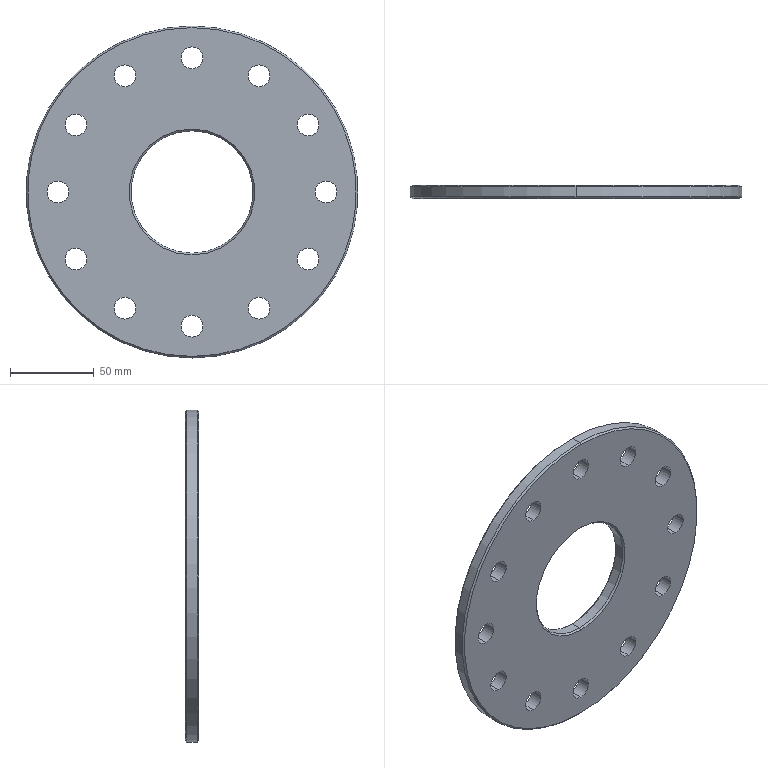Part | SolidWorks | features Chamfer 1, Extrusion 1 | 1 solid | 38 faces | box 198 x 8 x 198 mm | volume 199249 mm3 | cylinder 28 | cone 8 | plane 2 | commonest cylinder face diameters 13 x24 73 x2 198 x2
STEP:
#1=CARTESIAN_POINT('',(0.,79.,-98.));
#2=VERTEX_POINT('',#1);
#3=CARTESIAN_POINT('',(0.,79.,98.));
#4=VERTEX_POINT('',#3);
#5=CARTESIAN_POINT('',(0.,79.,0.));
#6=DIRECTION('',(0.,-1.,0.));
#7=DIRECTION('',(0.,0.,-1.));
#8=AXIS2_PLACEMENT_3D('',#5,#6,#7);
#9=CIRCLE('',#8,98.);
#10=EDGE_CURVE('',#2,#4,#9,.T.);
#11=ORIENTED_EDGE('',*,*,#10,.F.);
#12=CARTESIAN_POINT('',(0.,80.,-99.));
#13=VERTEX_POINT('',#12);
#14=CARTESIAN_POINT('',(0.,80.,-99.));
#15=DIRECTION('',(0.,0.7071,-0.7071));
#16=VECTOR('',#15,1000.);
#17=LINE('',#14,#16);
#18=EDGE_CURVE('',#2,#13,#17,.T.);
#19=ORIENTED_EDGE('',*,*,#18,.T.);
#20=CARTESIAN_POINT('',(0.,80.,99.));
#21=VERTEX_POINT('',#20);
#22=CARTESIAN_POINT('',(0.,80.,0.));
#23=DIRECTION('',(0.,1.,0.));
#24=DIRECTION('',(0.,0.,-1.));
#25=AXIS2_PLACEMENT_3D('',#22,#23,#24);
#26=CIRCLE('',#25,99.);
#27=EDGE_CURVE('',#21,#13,#26,.T.);
#28=ORIENTED_EDGE('',*,*,#27,.F.);
#29=CARTESIAN_POINT('',(0.,80.,99.));
#30=DIRECTION('',(0.,0.7071,0.7071));
#31=VECTOR('',#30,1000.);
#32=LINE('',#29,#31);
#33=EDGE_CURVE('',#4,#21,#32,.T.);
#34=ORIENTED_EDGE('',*,*,#33,.F.);
#35=EDGE_LOOP('',(#11,#19,#28,#34));
#36=FACE_OUTER_BOUND('',#35,.T.);
#37=CARTESIAN_POINT('',(0.,80.,0.));
#38=DIRECTION('',(0.,1.,0.));
#39=DIRECTION('',(0.,0.,1.));
#40=AXIS2_PLACEMENT_3D('',#37,#38,#39);
#41=CONICAL_SURFACE('',#40,99.,0.7854);
#42=ADVANCED_FACE('',(#36),#41,.T.);
#43=CARTESIAN_POINT('',(0.,87.,98.));
#44=VERTEX_POINT('',#43);
#45=CARTESIAN_POINT('',(0.,87.,-98.));
#46=VERTEX_POINT('',#45);
#47=CARTESIAN_POINT('',(0.,87.,0.));
#48=DIRECTION('',(0.,1.,0.));
#49=DIRECTION('',(0.,0.,-1.));
#50=AXIS2_PLACEMENT_3D('',#47,#48,#49);
#51=CIRCLE('',#50,98.);
#52=EDGE_CURVE('',#44,#46,#51,.T.);
#53=ORIENTED_EDGE('',*,*,#52,.F.);
#54=CARTESIAN_POINT('',(0.,86.,99.));
#55=VERTEX_POINT('',#54);
#56=CARTESIAN_POINT('',(0.,87.,98.));
#57=DIRECTION('',(0.,-0.7071,0.7071));
#58=VECTOR('',#57,1000.);
#59=LINE('',#56,#58);
#60=EDGE_CURVE('',#44,#55,#59,.T.);
#61=ORIENTED_EDGE('',*,*,#60,.T.);
#62=CARTESIAN_POINT('',(0.,86.,-99.));
#63=VERTEX_POINT('',#62);
#64=CARTESIAN_POINT('',(0.,86.,0.));
#65=DIRECTION('',(0.,-1.,0.));
#66=DIRECTION('',(0.,0.,-1.));
#67=AXIS2_PLACEMENT_3D('',#64,#65,#66);
#68=CIRCLE('',#67,99.);
#69=EDGE_CURVE('',#63,#55,#68,.T.);
#70=ORIENTED_EDGE('',*,*,#69,.F.);
#71=CARTESIAN_POINT('',(0.,87.,-98.));
#72=DIRECTION('',(0.,-0.7071,-0.7071));
#73=VECTOR('',#72,1000.);
#74=LINE('',#71,#73);
#75=EDGE_CURVE('',#46,#63,#74,.T.);
#76=ORIENTED_EDGE('',*,*,#75,.F.);
#77=EDGE_LOOP('',(#53,#61,#70,#76));
#78=FACE_OUTER_BOUND('',#77,.T.);
#79=CARTESIAN_POINT('',(0.,87.,0.));
#80=DIRECTION('',(0.,-1.,0.));
#81=DIRECTION('',(0.,0.,-1.));
#82=AXIS2_PLACEMENT_3D('',#79,#80,#81);
#83=CONICAL_SURFACE('',#82,98.,0.7854);
#84=ADVANCED_FACE('',(#78),#83,.T.);
#85=CARTESIAN_POINT('',(0.,80.,36.5));
#86=VERTEX_POINT('',#85);
#87=CARTESIAN_POINT('',(0.,80.,-36.5));
#88=VERTEX_POINT('',#87);
#89=CARTESIAN_POINT('',(0.,80.,0.));
#90=DIRECTION('',(0.,-1.,0.));
#91=DIRECTION('',(0.,0.,-1.));
#92=AXIS2_PLACEMENT_3D('',#89,#90,#91);
#93=CIRCLE('',#92,36.5);
#94=EDGE_CURVE('',#86,#88,#93,.T.);
#95=ORIENTED_EDGE('',*,*,#94,.F.);
#96=CARTESIAN_POINT('',(0.,79.,37.5));
#97=VERTEX_POINT('',#96);
#98=CARTESIAN_POINT('',(0.,79.,37.5));
#99=DIRECTION('',(0.,-0.7071,0.7071));
#100=VECTOR('',#99,1000.);
#101=LINE('',#98,#100);
#102=EDGE_CURVE('',#86,#97,#101,.T.);
#103=ORIENTED_EDGE('',*,*,#102,.T.);
#104=CARTESIAN_POINT('',(0.,79.,-37.5));
#105=VERTEX_POINT('',#104);
#106=CARTESIAN_POINT('',(0.,79.,0.));
#107=DIRECTION('',(0.,1.,0.));
#108=DIRECTION('',(0.,0.,-1.));
#109=AXIS2_PLACEMENT_3D('',#106,#107,#108);
#110=CIRCLE('',#109,37.5);
#111=EDGE_CURVE('',#105,#97,#110,.T.);
#112=ORIENTED_EDGE('',*,*,#111,.F.);
#113=CARTESIAN_POINT('',(0.,79.,-37.5));
#114=DIRECTION('',(0.,-0.7071,-0.7071));
#115=VECTOR('',#114,1000.);
#116=LINE('',#113,#115);
#117=EDGE_CURVE('',#88,#105,#116,.T.);
#118=ORIENTED_EDGE('',*,*,#117,.F.);
#119=EDGE_LOOP('',(#95,#103,#112,#118));
#120=FACE_OUTER_BOUND('',#119,.T.);
#121=CARTESIAN_POINT('',(0.,79.,0.));
#122=DIRECTION('',(0.,-1.,0.));
#123=DIRECTION('',(0.,0.,-1.));
#124=AXIS2_PLACEMENT_3D('',#121,#122,#123);
#125=CONICAL_SURFACE('',#124,37.5,0.7854);
#126=ADVANCED_FACE('',(#120),#125,.F.);
#127=CARTESIAN_POINT('',(0.,86.,-36.5));
#128=VERTEX_POINT('',#127);
#129=CARTESIAN_POINT('',(0.,86.,36.5));
#130=VERTEX_POINT('',#129);
#131=CARTESIAN_POINT('',(0.,86.,0.));
#132=DIRECTION('',(0.,1.,0.));
#133=DIRECTION('',(0.,0.,-1.));
#134=AXIS2_PLACEMENT_3D('',#131,#132,#133);
#135=CIRCLE('',#134,36.5);
#136=EDGE_CURVE('',#128,#130,#135,.T.);
#137=ORIENTED_EDGE('',*,*,#136,.F.);
#138=CARTESIAN_POINT('',(0.,87.,-37.5));
#139=VERTEX_POINT('',#138);
#140=CARTESIAN_POINT('',(0.,86.,-36.5));
#141=DIRECTION('',(0.,0.7071,-0.7071));
#142=VECTOR('',#141,1000.);
#143=LINE('',#140,#142);
#144=EDGE_CURVE('',#128,#139,#143,.T.);
#145=ORIENTED_EDGE('',*,*,#144,.T.);
#146=CARTESIAN_POINT('',(0.,87.,37.5));
#147=VERTEX_POINT('',#146);
#148=CARTESIAN_POINT('',(0.,87.,0.));
#149=DIRECTION('',(0.,-1.,0.));
#150=DIRECTION('',(0.,0.,-1.));
#151=AXIS2_PLACEMENT_3D('',#148,#149,#150);
#152=CIRCLE('',#151,37.5);
#153=EDGE_CURVE('',#147,#139,#152,.T.);
#154=ORIENTED_EDGE('',*,*,#153,.F.);
#155=CARTESIAN_POINT('',(0.,86.,36.5));
#156=DIRECTION('',(0.,0.7071,0.7071));
#157=VECTOR('',#156,1000.);
#158=LINE('',#155,#157);
#159=EDGE_CURVE('',#130,#147,#158,.T.);
#160=ORIENTED_EDGE('',*,*,#159,.F.);
#161=EDGE_LOOP('',(#137,#145,#154,#160));
#162=FACE_OUTER_BOUND('',#161,.T.);
#163=CARTESIAN_POINT('',(0.,86.,0.));
#164=DIRECTION('',(0.,1.,0.));
#165=DIRECTION('',(0.,0.,1.));
#166=AXIS2_PLACEMENT_3D('',#163,#164,#165);
#167=CONICAL_SURFACE('',#166,36.5,0.7854);
#168=ADVANCED_FACE('',(#162),#167,.F.);
#169=ORIENTED_EDGE('',*,*,#94,.T.);
#170=CARTESIAN_POINT('',(0.,79.,-36.5));
#171=DIRECTION('',(0.,1.,0.));
#172=VECTOR('',#171,1000.);
#173=LINE('',#170,#172);
#174=EDGE_CURVE('',#88,#128,#173,.T.);
#175=ORIENTED_EDGE('',*,*,#174,.T.);
#176=ORIENTED_EDGE('',*,*,#136,.T.);
#177=CARTESIAN_POINT('',(0.,79.,36.5));
#178=DIRECTION('',(0.,1.,0.));
#179=VECTOR('',#178,1000.);
#180=LINE('',#177,#179);
#181=EDGE_CURVE('',#86,#130,#180,.T.);
#182=ORIENTED_EDGE('',*,*,#181,.F.);
#183=EDGE_LOOP('',(#169,#175,#176,#182));
#184=FACE_OUTER_BOUND('',#183,.T.);
#185=CARTESIAN_POINT('',(0.,79.,0.));
#186=DIRECTION('',(0.,1.,0.));
#187=DIRECTION('',(0.,0.,1.));
#188=AXIS2_PLACEMENT_3D('',#185,#186,#187);
#189=CYLINDRICAL_SURFACE('',#188,36.5);
#190=ADVANCED_FACE('',(#184),#189,.F.);
#191=CARTESIAN_POINT('',(80.,79.,-6.5));
#192=VERTEX_POINT('',#191);
#193=CARTESIAN_POINT('',(80.,79.,6.5));
#194=VERTEX_POINT('',#193);
#195=CARTESIAN_POINT('',(80.,79.,0.));
#196=DIRECTION('',(0.,1.,0.));
#197=DIRECTION('',(0.,0.,-1.));
#198=AXIS2_PLACEMENT_3D('',#195,#196,#197);
#199=CIRCLE('',#198,6.5);
#200=EDGE_CURVE('',#192,#194,#199,.T.);
#201=ORIENTED_EDGE('',*,*,#200,.F.);
#202=CARTESIAN_POINT('',(80.,87.,-6.5));
#203=VERTEX_POINT('',#202);
#204=CARTESIAN_POINT('',(80.,79.,-6.5));
#205=DIRECTION('',(0.,1.,0.));
#206=VECTOR('',#205,1000.);
#207=LINE('',#204,#206);
#208=EDGE_CURVE('',#192,#203,#207,.T.);
#209=ORIENTED_EDGE('',*,*,#208,.T.);
#210=CARTESIAN_POINT('',(80.,87.,6.5));
#211=VERTEX_POINT('',#210);
#212=CARTESIAN_POINT('',(80.,87.,0.));
#213=DIRECTION('',(0.,1.,0.));
#214=DIRECTION('',(0.,0.,-1.));
#215=AXIS2_PLACEMENT_3D('',#212,#213,#214);
#216=CIRCLE('',#215,6.5);
#217=EDGE_CURVE('',#203,#211,#216,.T.);
#218=ORIENTED_EDGE('',*,*,#217,.T.);
#219=CARTESIAN_POINT('',(80.,79.,6.5));
#220=DIRECTION('',(0.,1.,0.));
#221=VECTOR('',#220,1000.);
#222=LINE('',#219,#221);
#223=EDGE_CURVE('',#194,#211,#222,.T.);
#224=ORIENTED_EDGE('',*,*,#223,.F.);
#225=EDGE_LOOP('',(#201,#209,#218,#224));
#226=FACE_OUTER_BOUND('',#225,.T.);
#227=CARTESIAN_POINT('',(80.,79.,0.));
#228=DIRECTION('',(0.,1.,0.));
#229=DIRECTION('',(0.,0.,1.));
#230=AXIS2_PLACEMENT_3D('',#227,#228,#229);
#231=CYLINDRICAL_SURFACE('',#230,6.5);
#232=ADVANCED_FACE('',(#226),#231,.F.);
#233=CARTESIAN_POINT('',(-40.,79.,62.782));
#234=VERTEX_POINT('',#233);
#235=CARTESIAN_POINT('',(-40.,79.,75.782));
#236=VERTEX_POINT('',#235);
#237=CARTESIAN_POINT('',(-40.,79.,69.282));
#238=DIRECTION('',(0.,1.,0.));
#239=DIRECTION('',(0.,0.,-1.));
#240=AXIS2_PLACEMENT_3D('',#237,#238,#239);
#241=CIRCLE('',#240,6.5);
#242=EDGE_CURVE('',#234,#236,#241,.T.);
#243=ORIENTED_EDGE('',*,*,#242,.F.);
#244=CARTESIAN_POINT('',(-40.,87.,62.782));
#245=VERTEX_POINT('',#244);
#246=CARTESIAN_POINT('',(-40.,79.,62.782));
#247=DIRECTION('',(0.,1.,0.));
#248=VECTOR('',#247,1000.);
#249=LINE('',#246,#248);
#250=EDGE_CURVE('',#234,#245,#249,.T.);
#251=ORIENTED_EDGE('',*,*,#250,.T.);
#252=CARTESIAN_POINT('',(-40.,87.,75.782));
#253=VERTEX_POINT('',#252);
#254=CARTESIAN_POINT('',(-40.,87.,69.282));
#255=DIRECTION('',(0.,1.,0.));
#256=DIRECTION('',(0.,0.,-1.));
#257=AXIS2_PLACEMENT_3D('',#254,#255,#256);
#258=CIRCLE('',#257,6.5);
#259=EDGE_CURVE('',#245,#253,#258,.T.);
#260=ORIENTED_EDGE('',*,*,#259,.T.);
#261=CARTESIAN_POINT('',(-40.,79.,75.782));
#262=DIRECTION('',(0.,1.,0.));
#263=VECTOR('',#262,1000.);
#264=LINE('',#261,#263);
#265=EDGE_CURVE('',#236,#253,#264,.T.);
#266=ORIENTED_EDGE('',*,*,#265,.F.);
#267=EDGE_LOOP('',(#243,#251,#260,#266));
#268=FACE_OUTER_BOUND('',#267,.T.);
#269=CARTESIAN_POINT('',(-40.,79.,69.282));
#270=DIRECTION('',(0.,1.,0.));
#271=DIRECTION('',(0.,0.,1.));
#272=AXIS2_PLACEMENT_3D('',#269,#270,#271);
#273=CYLINDRICAL_SURFACE('',#272,6.5);
#274=ADVANCED_FACE('',(#268),#273,.F.);
#275=CARTESIAN_POINT('',(69.282,79.,-46.5));
#276=VERTEX_POINT('',#275);
#277=CARTESIAN_POINT('',(69.282,79.,-33.5));
#278=VERTEX_POINT('',#277);
#279=CARTESIAN_POINT('',(69.282,79.,-40.));
#280=DIRECTION('',(0.,1.,0.));
#281=DIRECTION('',(0.,0.,-1.));
#282=AXIS2_PLACEMENT_3D('',#279,#280,#281);
#283=CIRCLE('',#282,6.5);
#284=EDGE_CURVE('',#276,#278,#283,.T.);
#285=ORIENTED_EDGE('',*,*,#284,.F.);
#286=CARTESIAN_POINT('',(69.282,87.,-46.5));
#287=VERTEX_POINT('',#286);
#288=CARTESIAN_POINT('',(69.282,79.,-46.5));
#289=DIRECTION('',(0.,1.,0.));
#290=VECTOR('',#289,1000.);
#291=LINE('',#288,#290);
#292=EDGE_CURVE('',#276,#287,#291,.T.);
#293=ORIENTED_EDGE('',*,*,#292,.T.);
#294=CARTESIAN_POINT('',(69.282,87.,-33.5));
#295=VERTEX_POINT('',#294);
#296=CARTESIAN_POINT('',(69.282,87.,-40.));
#297=DIRECTION('',(0.,1.,0.));
#298=DIRECTION('',(0.,0.,-1.));
#299=AXIS2_PLACEMENT_3D('',#296,#297,#298);
#300=CIRCLE('',#299,6.5);
#301=EDGE_CURVE('',#287,#295,#300,.T.);
#302=ORIENTED_EDGE('',*,*,#301,.T.);
#303=CARTESIAN_POINT('',(69.282,79.,-33.5));
#304=DIRECTION('',(0.,1.,0.));
#305=VECTOR('',#304,1000.);
#306=LINE('',#303,#305);
#307=EDGE_CURVE('',#278,#295,#306,.T.);
#308=ORIENTED_EDGE('',*,*,#307,.F.);
#309=EDGE_LOOP('',(#285,#293,#302,#308));
#310=FACE_OUTER_BOUND('',#309,.T.);
#311=CARTESIAN_POINT('',(69.282,79.,-40.));
#312=DIRECTION('',(0.,1.,0.));
#313=DIRECTION('',(0.,0.,1.));
#314=AXIS2_PLACEMENT_3D('',#311,#312,#313);
#315=CYLINDRICAL_SURFACE('',#314,6.5);
#316=ADVANCED_FACE('',(#310),#315,.F.);
#317=CARTESIAN_POINT('',(40.,79.,62.782));
#318=VERTEX_POINT('',#317);
#319=CARTESIAN_POINT('',(40.,79.,75.782));
#320=VERTEX_POINT('',#319);
#321=CARTESIAN_POINT('',(40.,79.,69.282));
#322=DIRECTION('',(0.,1.,0.));
#323=DIRECTION('',(0.,0.,-1.));
#324=AXIS2_PLACEMENT_3D('',#321,#322,#323);
#325=CIRCLE('',#324,6.5);
#326=EDGE_CURVE('',#318,#320,#325,.T.);
#327=ORIENTED_EDGE('',*,*,#326,.F.);
#328=CARTESIAN_POINT('',(40.,87.,62.782));
#329=VERTEX_POINT('',#328);
#330=CARTESIAN_POINT('',(40.,79.,62.782));
#331=DIRECTION('',(0.,1.,0.));
#332=VECTOR('',#331,1000.);
#333=LINE('',#330,#332);
#334=EDGE_CURVE('',#318,#329,#333,.T.);
#335=ORIENTED_EDGE('',*,*,#334,.T.);
#336=CARTESIAN_POINT('',(40.,87.,75.782));
#337=VERTEX_POINT('',#336);
#338=CARTESIAN_POINT('',(40.,87.,69.282));
#339=DIRECTION('',(0.,1.,0.));
#340=DIRECTION('',(0.,0.,-1.));
#341=AXIS2_PLACEMENT_3D('',#338,#339,#340);
#342=CIRCLE('',#341,6.5);
#343=EDGE_CURVE('',#329,#337,#342,.T.);
#344=ORIENTED_EDGE('',*,*,#343,.T.);
#345=CARTESIAN_POINT('',(40.,79.,75.782));
#346=DIRECTION('',(0.,1.,0.));
#347=VECTOR('',#346,1000.);
#348=LINE('',#345,#347);
#349=EDGE_CURVE('',#320,#337,#348,.T.);
#350=ORIENTED_EDGE('',*,*,#349,.F.);
#351=EDGE_LOOP('',(#327,#335,#344,#350));
#352=FACE_OUTER_BOUND('',#351,.T.);
#353=CARTESIAN_POINT('',(40.,79.,69.282));
#354=DIRECTION('',(0.,1.,0.));
#355=DIRECTION('',(0.,0.,1.));
#356=AXIS2_PLACEMENT_3D('',#353,#354,#355);
#357=CYLINDRICAL_SURFACE('',#356,6.5);
#358=ADVANCED_FACE('',(#352),#357,.F.);
#359=CARTESIAN_POINT('',(0.,79.,73.5));
#360=VERTEX_POINT('',#359);
#361=CARTESIAN_POINT('',(0.,79.,86.5));
#362=VERTEX_POINT('',#361);
#363=CARTESIAN_POINT('',(0.,79.,80.));
#364=DIRECTION('',(0.,1.,0.));
#365=DIRECTION('',(0.,0.,-1.));
#366=AXIS2_PLACEMENT_3D('',#363,#364,#365);
#367=CIRCLE('',#366,6.5);
#368=EDGE_CURVE('',#360,#362,#367,.T.);
#369=ORIENTED_EDGE('',*,*,#368,.F.);
#370=CARTESIAN_POINT('',(0.,87.,73.5));
#371=VERTEX_POINT('',#370);
#372=CARTESIAN_POINT('',(0.,79.,73.5));
#373=DIRECTION('',(0.,1.,0.));
#374=VECTOR('',#373,1000.);
#375=LINE('',#372,#374);
#376=EDGE_CURVE('',#360,#371,#375,.T.);
#377=ORIENTED_EDGE('',*,*,#376,.T.);
#378=CARTESIAN_POINT('',(0.,87.,86.5));
#379=VERTEX_POINT('',#378);
#380=CARTESIAN_POINT('',(0.,87.,80.));
#381=DIRECTION('',(0.,1.,0.));
#382=DIRECTION('',(0.,0.,-1.));
#383=AXIS2_PLACEMENT_3D('',#380,#381,#382);
#384=CIRCLE('',#383,6.5);
#385=EDGE_CURVE('',#371,#379,#384,.T.);
#386=ORIENTED_EDGE('',*,*,#385,.T.);
#387=CARTESIAN_POINT('',(0.,79.,86.5));
#388=DIRECTION('',(0.,1.,0.));
#389=VECTOR('',#388,1000.);
#390=LINE('',#387,#389);
#391=EDGE_CURVE('',#362,#379,#390,.T.);
#392=ORIENTED_EDGE('',*,*,#391,.F.);
#393=EDGE_LOOP('',(#369,#377,#386,#392));
#394=FACE_OUTER_BOUND('',#393,.T.);
#395=CARTESIAN_POINT('',(0.,79.,80.));
#396=DIRECTION('',(0.,1.,0.));
#397=DIRECTION('',(0.,0.,1.));
#398=AXIS2_PLACEMENT_3D('',#395,#396,#397);
#399=CYLINDRICAL_SURFACE('',#398,6.5);
#400=ADVANCED_FACE('',(#394),#399,.F.);
#401=CARTESIAN_POINT('',(-40.,79.,-75.782));
#402=VERTEX_POINT('',#401);
#403=CARTESIAN_POINT('',(-40.,79.,-62.782));
#404=VERTEX_POINT('',#403);
#405=CARTESIAN_POINT('',(-40.,79.,-69.282));
#406=DIRECTION('',(0.,1.,0.));
#407=DIRECTION('',(0.,0.,-1.));
#408=AXIS2_PLACEMENT_3D('',#405,#406,#407);
#409=CIRCLE('',#408,6.5);
#410=EDGE_CURVE('',#402,#404,#409,.T.);
#411=ORIENTED_EDGE('',*,*,#410,.F.);
#412=CARTESIAN_POINT('',(-40.,87.,-75.782));
#413=VERTEX_POINT('',#412);
#414=CARTESIAN_POINT('',(-40.,79.,-75.782));
#415=DIRECTION('',(0.,1.,0.));
#416=VECTOR('',#415,1000.);
#417=LINE('',#414,#416);
#418=EDGE_CURVE('',#402,#413,#417,.T.);
#419=ORIENTED_EDGE('',*,*,#418,.T.);
#420=CARTESIAN_POINT('',(-40.,87.,-62.782));
#421=VERTEX_POINT('',#420);
#422=CARTESIAN_POINT('',(-40.,87.,-69.282));
#423=DIRECTION('',(0.,1.,0.));
#424=DIRECTION('',(0.,0.,-1.));
#425=AXIS2_PLACEMENT_3D('',#422,#423,#424);
#426=CIRCLE('',#425,6.5);
#427=EDGE_CURVE('',#413,#421,#426,.T.);
#428=ORIENTED_EDGE('',*,*,#427,.T.);
#429=CARTESIAN_POINT('',(-40.,79.,-62.782));
#430=DIRECTION('',(0.,1.,0.));
#431=VECTOR('',#430,1000.);
#432=LINE('',#429,#431);
#433=EDGE_CURVE('',#404,#421,#432,.T.);
#434=ORIENTED_EDGE('',*,*,#433,.F.);
#435=EDGE_LOOP('',(#411,#419,#428,#434));
#436=FACE_OUTER_BOUND('',#435,.T.);
#437=CARTESIAN_POINT('',(-40.,79.,-69.282));
#438=DIRECTION('',(0.,1.,0.));
#439=DIRECTION('',(0.,0.,1.));
#440=AXIS2_PLACEMENT_3D('',#437,#438,#439);
#441=CYLINDRICAL_SURFACE('',#440,6.5);
#442=ADVANCED_FACE('',(#436),#441,.F.);
#443=CARTESIAN_POINT('',(69.282,79.,33.5));
#444=VERTEX_POINT('',#443);
#445=CARTESIAN_POINT('',(69.282,79.,46.5));
#446=VERTEX_POINT('',#445);
#447=CARTESIAN_POINT('',(69.282,79.,40.));
#448=DIRECTION('',(0.,1.,0.));
#449=DIRECTION('',(0.,0.,-1.));
#450=AXIS2_PLACEMENT_3D('',#447,#448,#449);
#451=CIRCLE('',#450,6.5);
#452=EDGE_CURVE('',#444,#446,#451,.T.);
#453=ORIENTED_EDGE('',*,*,#452,.F.);
#454=CARTESIAN_POINT('',(69.282,87.,33.5));
#455=VERTEX_POINT('',#454);
#456=CARTESIAN_POINT('',(69.282,79.,33.5));
#457=DIRECTION('',(0.,1.,0.));
#458=VECTOR('',#457,1000.);
#459=LINE('',#456,#458);
#460=EDGE_CURVE('',#444,#455,#459,.T.);
#461=ORIENTED_EDGE('',*,*,#460,.T.);
#462=CARTESIAN_POINT('',(69.282,87.,46.5));
#463=VERTEX_POINT('',#462);
#464=CARTESIAN_POINT('',(69.282,87.,40.));
#465=DIRECTION('',(0.,1.,0.));
#466=DIRECTION('',(0.,0.,-1.));
#467=AXIS2_PLACEMENT_3D('',#464,#465,#466);
#468=CIRCLE('',#467,6.5);
#469=EDGE_CURVE('',#455,#463,#468,.T.);
#470=ORIENTED_EDGE('',*,*,#469,.T.);
#471=CARTESIAN_POINT('',(69.282,79.,46.5));
#472=DIRECTION('',(0.,1.,0.));
#473=VECTOR('',#472,1000.);
#474=LINE('',#471,#473);
#475=EDGE_CURVE('',#446,#463,#474,.T.);
#476=ORIENTED_EDGE('',*,*,#475,.F.);
#477=EDGE_LOOP('',(#453,#461,#470,#476));
#478=FACE_OUTER_BOUND('',#477,.T.);
#479=CARTESIAN_POINT('',(69.282,79.,40.));
#480=DIRECTION('',(0.,1.,0.));
#481=DIRECTION('',(0.,0.,1.));
#482=AXIS2_PLACEMENT_3D('',#479,#480,#481);
#483=CYLINDRICAL_SURFACE('',#482,6.5);
#484=ADVANCED_FACE('',(#478),#483,.F.);
#485=CARTESIAN_POINT('',(0.,79.,-86.5));
#486=VERTEX_POINT('',#485);
#487=CARTESIAN_POINT('',(0.,79.,-73.5));
#488=VERTEX_POINT('',#487);
#489=CARTESIAN_POINT('',(0.,79.,-80.));
#490=DIRECTION('',(0.,1.,0.));
#491=DIRECTION('',(0.,0.,-1.));
#492=AXIS2_PLACEMENT_3D('',#489,#490,#491);
#493=CIRCLE('',#492,6.5);
#494=EDGE_CURVE('',#486,#488,#493,.T.);
#495=ORIENTED_EDGE('',*,*,#494,.F.);
#496=CARTESIAN_POINT('',(0.,87.,-86.5));
#497=VERTEX_POINT('',#496);
#498=CARTESIAN_POINT('',(0.,79.,-86.5));
#499=DIRECTION('',(0.,1.,0.));
#500=VECTOR('',#499,1000.);
#501=LINE('',#498,#500);
#502=EDGE_CURVE('',#486,#497,#501,.T.);
#503=ORIENTED_EDGE('',*,*,#502,.T.);
#504=CARTESIAN_POINT('',(0.,87.,-73.5));
#505=VERTEX_POINT('',#504);
#506=CARTESIAN_POINT('',(0.,87.,-80.));
#507=DIRECTION('',(0.,1.,0.));
#508=DIRECTION('',(0.,0.,-1.));
#509=AXIS2_PLACEMENT_3D('',#506,#507,#508);
#510=CIRCLE('',#509,6.5);
#511=EDGE_CURVE('',#497,#505,#510,.T.);
#512=ORIENTED_EDGE('',*,*,#511,.T.);
#513=CARTESIAN_POINT('',(0.,79.,-73.5));
#514=DIRECTION('',(0.,1.,0.));
#515=VECTOR('',#514,1000.);
#516=LINE('',#513,#515);
#517=EDGE_CURVE('',#488,#505,#516,.T.);
#518=ORIENTED_EDGE('',*,*,#517,.F.);
#519=EDGE_LOOP('',(#495,#503,#512,#518));
#520=FACE_OUTER_BOUND('',#519,.T.);
#521=CARTESIAN_POINT('',(0.,79.,-80.));
#522=DIRECTION('',(0.,1.,0.));
#523=DIRECTION('',(0.,0.,1.));
#524=AXIS2_PLACEMENT_3D('',#521,#522,#523);
#525=CYLINDRICAL_SURFACE('',#524,6.5);
#526=ADVANCED_FACE('',(#520),#525,.F.);
#527=CARTESIAN_POINT('',(-69.282,79.,33.5));
#528=VERTEX_POINT('',#527);
#529=CARTESIAN_POINT('',(-69.282,79.,46.5));
#530=VERTEX_POINT('',#529);
#531=CARTESIAN_POINT('',(-69.282,79.,40.));
#532=DIRECTION('',(0.,1.,0.));
#533=DIRECTION('',(0.,0.,-1.));
#534=AXIS2_PLACEMENT_3D('',#531,#532,#533);
#535=CIRCLE('',#534,6.5);
#536=EDGE_CURVE('',#528,#530,#535,.T.);
#537=ORIENTED_EDGE('',*,*,#536,.F.);
#538=CARTESIAN_POINT('',(-69.282,87.,33.5));
#539=VERTEX_POINT('',#538);
#540=CARTESIAN_POINT('',(-69.282,79.,33.5));
#541=DIRECTION('',(0.,1.,0.));
#542=VECTOR('',#541,1000.);
#543=LINE('',#540,#542);
#544=EDGE_CURVE('',#528,#539,#543,.T.);
#545=ORIENTED_EDGE('',*,*,#544,.T.);
#546=CARTESIAN_POINT('',(-69.282,87.,46.5));
#547=VERTEX_POINT('',#546);
#548=CARTESIAN_POINT('',(-69.282,87.,40.));
#549=DIRECTION('',(0.,1.,0.));
#550=DIRECTION('',(0.,0.,-1.));
#551=AXIS2_PLACEMENT_3D('',#548,#549,#550);
#552=CIRCLE('',#551,6.5);
#553=EDGE_CURVE('',#539,#547,#552,.T.);
#554=ORIENTED_EDGE('',*,*,#553,.T.);
#555=CARTESIAN_POINT('',(-69.282,79.,46.5));
#556=DIRECTION('',(0.,1.,0.));
#557=VECTOR('',#556,1000.);
#558=LINE('',#555,#557);
#559=EDGE_CURVE('',#530,#547,#558,.T.);
#560=ORIENTED_EDGE('',*,*,#559,.F.);
#561=EDGE_LOOP('',(#537,#545,#554,#560));
#562=FACE_OUTER_BOUND('',#561,.T.);
#563=CARTESIAN_POINT('',(-69.282,79.,40.));
#564=DIRECTION('',(0.,1.,0.));
#565=DIRECTION('',(0.,0.,1.));
#566=AXIS2_PLACEMENT_3D('',#563,#564,#565);
#567=CYLINDRICAL_SURFACE('',#566,6.5);
#568=ADVANCED_FACE('',(#562),#567,.F.);
#569=CARTESIAN_POINT('',(-69.282,79.,-46.5));
#570=VERTEX_POINT('',#569);
#571=CARTESIAN_POINT('',(-69.282,79.,-33.5));
#572=VERTEX_POINT('',#571);
#573=CARTESIAN_POINT('',(-69.282,79.,-40.));
#574=DIRECTION('',(0.,1.,0.));
#575=DIRECTION('',(0.,0.,-1.));
#576=AXIS2_PLACEMENT_3D('',#573,#574,#575);
#577=CIRCLE('',#576,6.5);
#578=EDGE_CURVE('',#570,#572,#577,.T.);
#579=ORIENTED_EDGE('',*,*,#578,.F.);
#580=CARTESIAN_POINT('',(-69.282,87.,-46.5));
#581=VERTEX_POINT('',#580);
#582=CARTESIAN_POINT('',(-69.282,79.,-46.5));
#583=DIRECTION('',(0.,1.,0.));
#584=VECTOR('',#583,1000.);
#585=LINE('',#582,#584);
#586=EDGE_CURVE('',#570,#581,#585,.T.);
#587=ORIENTED_EDGE('',*,*,#586,.T.);
#588=CARTESIAN_POINT('',(-69.282,87.,-33.5));
#589=VERTEX_POINT('',#588);
#590=CARTESIAN_POINT('',(-69.282,87.,-40.));
#591=DIRECTION('',(0.,1.,0.));
#592=DIRECTION('',(0.,0.,-1.));
#593=AXIS2_PLACEMENT_3D('',#590,#591,#592);
#594=CIRCLE('',#593,6.5);
#595=EDGE_CURVE('',#581,#589,#594,.T.);
#596=ORIENTED_EDGE('',*,*,#595,.T.);
#597=CARTESIAN_POINT('',(-69.282,79.,-33.5));
#598=DIRECTION('',(0.,1.,0.));
#599=VECTOR('',#598,1000.);
#600=LINE('',#597,#599);
#601=EDGE_CURVE('',#572,#589,#600,.T.);
#602=ORIENTED_EDGE('',*,*,#601,.F.);
#603=EDGE_LOOP('',(#579,#587,#596,#602));
#604=FACE_OUTER_BOUND('',#603,.T.);
#605=CARTESIAN_POINT('',(-69.282,79.,-40.));
#606=DIRECTION('',(0.,1.,0.));
#607=DIRECTION('',(0.,0.,1.));
#608=AXIS2_PLACEMENT_3D('',#605,#606,#607);
#609=CYLINDRICAL_SURFACE('',#608,6.5);
#610=ADVANCED_FACE('',(#604),#609,.F.);
#611=CARTESIAN_POINT('',(40.,79.,-75.782));
#612=VERTEX_POINT('',#611);
#613=CARTESIAN_POINT('',(40.,79.,-62.782));
#614=VERTEX_POINT('',#613);
#615=CARTESIAN_POINT('',(40.,79.,-69.282));
#616=DIRECTION('',(0.,1.,0.));
#617=DIRECTION('',(0.,0.,-1.));
#618=AXIS2_PLACEMENT_3D('',#615,#616,#617);
#619=CIRCLE('',#618,6.5);
#620=EDGE_CURVE('',#612,#614,#619,.T.);
#621=ORIENTED_EDGE('',*,*,#620,.F.);
#622=CARTESIAN_POINT('',(40.,87.,-75.782));
#623=VERTEX_POINT('',#622);
#624=CARTESIAN_POINT('',(40.,79.,-75.782));
#625=DIRECTION('',(0.,1.,0.));
#626=VECTOR('',#625,1000.);
#627=LINE('',#624,#626);
#628=EDGE_CURVE('',#612,#623,#627,.T.);
#629=ORIENTED_EDGE('',*,*,#628,.T.);
#630=CARTESIAN_POINT('',(40.,87.,-62.782));
#631=VERTEX_POINT('',#630);
#632=CARTESIAN_POINT('',(40.,87.,-69.282));
#633=DIRECTION('',(0.,1.,0.));
#634=DIRECTION('',(0.,0.,-1.));
#635=AXIS2_PLACEMENT_3D('',#632,#633,#634);
#636=CIRCLE('',#635,6.5);
#637=EDGE_CURVE('',#623,#631,#636,.T.);
#638=ORIENTED_EDGE('',*,*,#637,.T.);
#639=CARTESIAN_POINT('',(40.,79.,-62.782));
#640=DIRECTION('',(0.,1.,0.));
#641=VECTOR('',#640,1000.);
#642=LINE('',#639,#641);
#643=EDGE_CURVE('',#614,#631,#642,.T.);
#644=ORIENTED_EDGE('',*,*,#643,.F.);
#645=EDGE_LOOP('',(#621,#629,#638,#644));
#646=FACE_OUTER_BOUND('',#645,.T.);
#647=CARTESIAN_POINT('',(40.,79.,-69.282));
#648=DIRECTION('',(0.,1.,0.));
#649=DIRECTION('',(0.,0.,1.));
#650=AXIS2_PLACEMENT_3D('',#647,#648,#649);
#651=CYLINDRICAL_SURFACE('',#650,6.5);
#652=ADVANCED_FACE('',(#646),#651,.F.);
#653=CARTESIAN_POINT('',(-80.,79.,-6.5));
#654=VERTEX_POINT('',#653);
#655=CARTESIAN_POINT('',(-80.,79.,6.5));
#656=VERTEX_POINT('',#655);
#657=CARTESIAN_POINT('',(-80.,79.,0.));
#658=DIRECTION('',(0.,1.,0.));
#659=DIRECTION('',(0.,0.,-1.));
#660=AXIS2_PLACEMENT_3D('',#657,#658,#659);
#661=CIRCLE('',#660,6.5);
#662=EDGE_CURVE('',#654,#656,#661,.T.);
#663=ORIENTED_EDGE('',*,*,#662,.F.);
#664=CARTESIAN_POINT('',(-80.,87.,-6.5));
#665=VERTEX_POINT('',#664);
#666=CARTESIAN_POINT('',(-80.,79.,-6.5));
#667=DIRECTION('',(0.,1.,0.));
#668=VECTOR('',#667,1000.);
#669=LINE('',#666,#668);
#670=EDGE_CURVE('',#654,#665,#669,.T.);
#671=ORIENTED_EDGE('',*,*,#670,.T.);
#672=CARTESIAN_POINT('',(-80.,87.,6.5));
#673=VERTEX_POINT('',#672);
#674=CARTESIAN_POINT('',(-80.,87.,0.));
#675=DIRECTION('',(0.,1.,0.));
#676=DIRECTION('',(0.,0.,-1.));
#677=AXIS2_PLACEMENT_3D('',#674,#675,#676);
#678=CIRCLE('',#677,6.5);
#679=EDGE_CURVE('',#665,#673,#678,.T.);
#680=ORIENTED_EDGE('',*,*,#679,.T.);
#681=CARTESIAN_POINT('',(-80.,79.,6.5));
#682=DIRECTION('',(0.,1.,0.));
#683=VECTOR('',#682,1000.);
#684=LINE('',#681,#683);
#685=EDGE_CURVE('',#656,#673,#684,.T.);
#686=ORIENTED_EDGE('',*,*,#685,.F.);
#687=EDGE_LOOP('',(#663,#671,#680,#686));
#688=FACE_OUTER_BOUND('',#687,.T.);
#689=CARTESIAN_POINT('',(-80.,79.,0.));
#690=DIRECTION('',(0.,1.,0.));
#691=DIRECTION('',(0.,0.,1.));
#692=AXIS2_PLACEMENT_3D('',#689,#690,#691);
#693=CYLINDRICAL_SURFACE('',#692,6.5);
#694=ADVANCED_FACE('',(#688),#693,.F.);
#695=ORIENTED_EDGE('',*,*,#27,.T.);
#696=CARTESIAN_POINT('',(0.,79.,-99.));
#697=DIRECTION('',(0.,1.,0.));
#698=VECTOR('',#697,1000.);
#699=LINE('',#696,#698);
#700=EDGE_CURVE('',#13,#63,#699,.T.);
#701=ORIENTED_EDGE('',*,*,#700,.T.);
#702=ORIENTED_EDGE('',*,*,#69,.T.);
#703=CARTESIAN_POINT('',(0.,79.,99.));
#704=DIRECTION('',(0.,1.,0.));
#705=VECTOR('',#704,1000.);
#706=LINE('',#703,#705);
#707=EDGE_CURVE('',#21,#55,#706,.T.);
#708=ORIENTED_EDGE('',*,*,#707,.F.);
#709=EDGE_LOOP('',(#695,#701,#702,#708));
#710=FACE_OUTER_BOUND('',#709,.T.);
#711=CARTESIAN_POINT('',(0.,79.,0.));
#712=DIRECTION('',(0.,1.,0.));
#713=DIRECTION('',(0.,0.,1.));
#714=AXIS2_PLACEMENT_3D('',#711,#712,#713);
#715=CYLINDRICAL_SURFACE('',#714,99.);
#716=ADVANCED_FACE('',(#710),#715,.T.);
#717=ORIENTED_EDGE('',*,*,#700,.F.);
#718=CARTESIAN_POINT('',(0.,80.,0.));
#719=DIRECTION('',(0.,1.,0.));
#720=DIRECTION('',(0.,0.,-1.));
#721=AXIS2_PLACEMENT_3D('',#718,#719,#720);
#722=CIRCLE('',#721,99.);
#723=EDGE_CURVE('',#13,#21,#722,.T.);
#724=ORIENTED_EDGE('',*,*,#723,.T.);
#725=ORIENTED_EDGE('',*,*,#707,.T.);
#726=CARTESIAN_POINT('',(0.,86.,0.));
#727=DIRECTION('',(0.,-1.,0.));
#728=DIRECTION('',(0.,0.,-1.));
#729=AXIS2_PLACEMENT_3D('',#726,#727,#728);
#730=CIRCLE('',#729,99.);
#731=EDGE_CURVE('',#55,#63,#730,.T.);
#732=ORIENTED_EDGE('',*,*,#731,.T.);
#733=EDGE_LOOP('',(#717,#724,#725,#732));
#734=FACE_OUTER_BOUND('',#733,.T.);
#735=CARTESIAN_POINT('',(0.,79.,0.));
#736=DIRECTION('',(0.,1.,0.));
#737=DIRECTION('',(0.,0.,1.));
#738=AXIS2_PLACEMENT_3D('',#735,#736,#737);
#739=CYLINDRICAL_SURFACE('',#738,99.);
#740=ADVANCED_FACE('',(#734),#739,.T.);
#741=ORIENTED_EDGE('',*,*,#111,.T.);
#742=CARTESIAN_POINT('',(0.,79.,0.));
#743=DIRECTION('',(0.,1.,0.));
#744=DIRECTION('',(0.,0.,-1.));
#745=AXIS2_PLACEMENT_3D('',#742,#743,#744);
#746=CIRCLE('',#745,37.5);
#747=EDGE_CURVE('',#97,#105,#746,.T.);
#748=ORIENTED_EDGE('',*,*,#747,.T.);
#749=EDGE_LOOP('',(#741,#748));
#750=FACE_BOUND('',#749,.T.);
#751=CARTESIAN_POINT('',(0.,79.,0.));
#752=DIRECTION('',(0.,-1.,0.));
#753=DIRECTION('',(0.,0.,-1.));
#754=AXIS2_PLACEMENT_3D('',#751,#752,#753);
#755=CIRCLE('',#754,98.);
#756=EDGE_CURVE('',#4,#2,#755,.T.);
#757=ORIENTED_EDGE('',*,*,#756,.T.);
#758=ORIENTED_EDGE('',*,*,#10,.T.);
#759=EDGE_LOOP('',(#757,#758));
#760=FACE_OUTER_BOUND('',#759,.T.);
#761=CARTESIAN_POINT('',(80.,79.,0.));
#762=DIRECTION('',(0.,1.,0.));
#763=DIRECTION('',(0.,0.,-1.));
#764=AXIS2_PLACEMENT_3D('',#761,#762,#763);
#765=CIRCLE('',#764,6.5);
#766=EDGE_CURVE('',#194,#192,#765,.T.);
#767=ORIENTED_EDGE('',*,*,#766,.T.);
#768=ORIENTED_EDGE('',*,*,#200,.T.);
#769=EDGE_LOOP('',(#767,#768));
#770=FACE_BOUND('',#769,.T.);
#771=CARTESIAN_POINT('',(-40.,79.,69.282));
#772=DIRECTION('',(0.,1.,0.));
#773=DIRECTION('',(0.,0.,-1.));
#774=AXIS2_PLACEMENT_3D('',#771,#772,#773);
#775=CIRCLE('',#774,6.5);
#776=EDGE_CURVE('',#236,#234,#775,.T.);
#777=ORIENTED_EDGE('',*,*,#776,.T.);
#778=ORIENTED_EDGE('',*,*,#242,.T.);
#779=EDGE_LOOP('',(#777,#778));
#780=FACE_BOUND('',#779,.T.);
#781=CARTESIAN_POINT('',(69.282,79.,-40.));
#782=DIRECTION('',(0.,1.,0.));
#783=DIRECTION('',(0.,0.,-1.));
#784=AXIS2_PLACEMENT_3D('',#781,#782,#783);
#785=CIRCLE('',#784,6.5);
#786=EDGE_CURVE('',#278,#276,#785,.T.);
#787=ORIENTED_EDGE('',*,*,#786,.T.);
#788=ORIENTED_EDGE('',*,*,#284,.T.);
#789=EDGE_LOOP('',(#787,#788));
#790=FACE_BOUND('',#789,.T.);
#791=CARTESIAN_POINT('',(40.,79.,69.282));
#792=DIRECTION('',(0.,1.,0.));
#793=DIRECTION('',(0.,0.,-1.));
#794=AXIS2_PLACEMENT_3D('',#791,#792,#793);
#795=CIRCLE('',#794,6.5);
#796=EDGE_CURVE('',#320,#318,#795,.T.);
#797=ORIENTED_EDGE('',*,*,#796,.T.);
#798=ORIENTED_EDGE('',*,*,#326,.T.);
#799=EDGE_LOOP('',(#797,#798));
#800=FACE_BOUND('',#799,.T.);
#801=CARTESIAN_POINT('',(0.,79.,80.));
#802=DIRECTION('',(0.,1.,0.));
#803=DIRECTION('',(0.,0.,-1.));
#804=AXIS2_PLACEMENT_3D('',#801,#802,#803);
#805=CIRCLE('',#804,6.5);
#806=EDGE_CURVE('',#362,#360,#805,.T.);
#807=ORIENTED_EDGE('',*,*,#806,.T.);
#808=ORIENTED_EDGE('',*,*,#368,.T.);
#809=EDGE_LOOP('',(#807,#808));
#810=FACE_BOUND('',#809,.T.);
#811=CARTESIAN_POINT('',(-40.,79.,-69.282));
#812=DIRECTION('',(0.,1.,0.));
#813=DIRECTION('',(0.,0.,-1.));
#814=AXIS2_PLACEMENT_3D('',#811,#812,#813);
#815=CIRCLE('',#814,6.5);
#816=EDGE_CURVE('',#404,#402,#815,.T.);
#817=ORIENTED_EDGE('',*,*,#816,.T.);
#818=ORIENTED_EDGE('',*,*,#410,.T.);
#819=EDGE_LOOP('',(#817,#818));
#820=FACE_BOUND('',#819,.T.);
#821=CARTESIAN_POINT('',(69.282,79.,40.));
#822=DIRECTION('',(0.,1.,0.));
#823=DIRECTION('',(0.,0.,-1.));
#824=AXIS2_PLACEMENT_3D('',#821,#822,#823);
#825=CIRCLE('',#824,6.5);
#826=EDGE_CURVE('',#446,#444,#825,.T.);
#827=ORIENTED_EDGE('',*,*,#826,.T.);
#828=ORIENTED_EDGE('',*,*,#452,.T.);
#829=EDGE_LOOP('',(#827,#828));
#830=FACE_BOUND('',#829,.T.);
#831=CARTESIAN_POINT('',(0.,79.,-80.));
#832=DIRECTION('',(0.,1.,0.));
#833=DIRECTION('',(0.,0.,-1.));
#834=AXIS2_PLACEMENT_3D('',#831,#832,#833);
#835=CIRCLE('',#834,6.5);
#836=EDGE_CURVE('',#488,#486,#835,.T.);
#837=ORIENTED_EDGE('',*,*,#836,.T.);
#838=ORIENTED_EDGE('',*,*,#494,.T.);
#839=EDGE_LOOP('',(#837,#838));
#840=FACE_BOUND('',#839,.T.);
#841=CARTESIAN_POINT('',(-69.282,79.,40.));
#842=DIRECTION('',(0.,1.,0.));
#843=DIRECTION('',(0.,0.,-1.));
#844=AXIS2_PLACEMENT_3D('',#841,#842,#843);
#845=CIRCLE('',#844,6.5);
#846=EDGE_CURVE('',#530,#528,#845,.T.);
#847=ORIENTED_EDGE('',*,*,#846,.T.);
#848=ORIENTED_EDGE('',*,*,#536,.T.);
#849=EDGE_LOOP('',(#847,#848));
#850=FACE_BOUND('',#849,.T.);
#851=CARTESIAN_POINT('',(-69.282,79.,-40.));
#852=DIRECTION('',(0.,1.,0.));
#853=DIRECTION('',(0.,0.,-1.));
#854=AXIS2_PLACEMENT_3D('',#851,#852,#853);
#855=CIRCLE('',#854,6.5);
#856=EDGE_CURVE('',#572,#570,#855,.T.);
#857=ORIENTED_EDGE('',*,*,#856,.T.);
#858=ORIENTED_EDGE('',*,*,#578,.T.);
#859=EDGE_LOOP('',(#857,#858));
#860=FACE_BOUND('',#859,.T.);
#861=CARTESIAN_POINT('',(40.,79.,-69.282));
#862=DIRECTION('',(0.,1.,0.));
#863=DIRECTION('',(0.,0.,-1.));
#864=AXIS2_PLACEMENT_3D('',#861,#862,#863);
#865=CIRCLE('',#864,6.5);
#866=EDGE_CURVE('',#614,#612,#865,.T.);
#867=ORIENTED_EDGE('',*,*,#866,.T.);
#868=ORIENTED_EDGE('',*,*,#620,.T.);
#869=EDGE_LOOP('',(#867,#868));
#870=FACE_BOUND('',#869,.T.);
#871=CARTESIAN_POINT('',(-80.,79.,0.));
#872=DIRECTION('',(0.,1.,0.));
#873=DIRECTION('',(0.,0.,-1.));
#874=AXIS2_PLACEMENT_3D('',#871,#872,#873);
#875=CIRCLE('',#874,6.5);
#876=EDGE_CURVE('',#656,#654,#875,.T.);
#877=ORIENTED_EDGE('',*,*,#876,.T.);
#878=ORIENTED_EDGE('',*,*,#662,.T.);
#879=EDGE_LOOP('',(#877,#878));
#880=FACE_BOUND('',#879,.T.);
#881=CARTESIAN_POINT('',(0.,79.,0.));
#882=DIRECTION('',(0.,-1.,0.));
#883=DIRECTION('',(0.,0.,-1.));
#884=AXIS2_PLACEMENT_3D('',#881,#882,#883);
#885=PLANE('',#884);
#886=ADVANCED_FACE('',(#750,#760,#770,#780,#790,#800,#810,#820,#830,#840,#850,#860,#870,#880),#885,.T.);
#887=ORIENTED_EDGE('',*,*,#153,.T.);
#888=CARTESIAN_POINT('',(0.,87.,0.));
#889=DIRECTION('',(0.,-1.,0.));
#890=DIRECTION('',(0.,0.,-1.));
#891=AXIS2_PLACEMENT_3D('',#888,#889,#890);
#892=CIRCLE('',#891,37.5);
#893=EDGE_CURVE('',#139,#147,#892,.T.);
#894=ORIENTED_EDGE('',*,*,#893,.T.);
#895=EDGE_LOOP('',(#887,#894));
#896=FACE_BOUND('',#895,.T.);
#897=CARTESIAN_POINT('',(0.,87.,0.));
#898=DIRECTION('',(0.,1.,0.));
#899=DIRECTION('',(0.,0.,-1.));
#900=AXIS2_PLACEMENT_3D('',#897,#898,#899);
#901=CIRCLE('',#900,98.);
#902=EDGE_CURVE('',#46,#44,#901,.T.);
#903=ORIENTED_EDGE('',*,*,#902,.T.);
#904=ORIENTED_EDGE('',*,*,#52,.T.);
#905=EDGE_LOOP('',(#903,#904));
#906=FACE_OUTER_BOUND('',#905,.T.);
#907=CARTESIAN_POINT('',(80.,87.,0.));
#908=DIRECTION('',(0.,1.,0.));
#909=DIRECTION('',(0.,0.,-1.));
#910=AXIS2_PLACEMENT_3D('',#907,#908,#909);
#911=CIRCLE('',#910,6.5);
#912=EDGE_CURVE('',#211,#203,#911,.T.);
#913=ORIENTED_EDGE('',*,*,#912,.F.);
#914=ORIENTED_EDGE('',*,*,#217,.F.);
#915=EDGE_LOOP('',(#913,#914));
#916=FACE_BOUND('',#915,.T.);
#917=CARTESIAN_POINT('',(-40.,87.,69.282));
#918=DIRECTION('',(0.,1.,0.));
#919=DIRECTION('',(0.,0.,-1.));
#920=AXIS2_PLACEMENT_3D('',#917,#918,#919);
#921=CIRCLE('',#920,6.5);
#922=EDGE_CURVE('',#253,#245,#921,.T.);
#923=ORIENTED_EDGE('',*,*,#922,.F.);
#924=ORIENTED_EDGE('',*,*,#259,.F.);
#925=EDGE_LOOP('',(#923,#924));
#926=FACE_BOUND('',#925,.T.);
#927=CARTESIAN_POINT('',(69.282,87.,-40.));
#928=DIRECTION('',(0.,1.,0.));
#929=DIRECTION('',(0.,0.,-1.));
#930=AXIS2_PLACEMENT_3D('',#927,#928,#929);
#931=CIRCLE('',#930,6.5);
#932=EDGE_CURVE('',#295,#287,#931,.T.);
#933=ORIENTED_EDGE('',*,*,#932,.F.);
#934=ORIENTED_EDGE('',*,*,#301,.F.);
#935=EDGE_LOOP('',(#933,#934));
#936=FACE_BOUND('',#935,.T.);
#937=CARTESIAN_POINT('',(40.,87.,69.282));
#938=DIRECTION('',(0.,1.,0.));
#939=DIRECTION('',(0.,0.,-1.));
#940=AXIS2_PLACEMENT_3D('',#937,#938,#939);
#941=CIRCLE('',#940,6.5);
#942=EDGE_CURVE('',#337,#329,#941,.T.);
#943=ORIENTED_EDGE('',*,*,#942,.F.);
#944=ORIENTED_EDGE('',*,*,#343,.F.);
#945=EDGE_LOOP('',(#943,#944));
#946=FACE_BOUND('',#945,.T.);
#947=CARTESIAN_POINT('',(0.,87.,80.));
#948=DIRECTION('',(0.,1.,0.));
#949=DIRECTION('',(0.,0.,-1.));
#950=AXIS2_PLACEMENT_3D('',#947,#948,#949);
#951=CIRCLE('',#950,6.5);
#952=EDGE_CURVE('',#379,#371,#951,.T.);
#953=ORIENTED_EDGE('',*,*,#952,.F.);
#954=ORIENTED_EDGE('',*,*,#385,.F.);
#955=EDGE_LOOP('',(#953,#954));
#956=FACE_BOUND('',#955,.T.);
#957=CARTESIAN_POINT('',(-40.,87.,-69.282));
#958=DIRECTION('',(0.,1.,0.));
#959=DIRECTION('',(0.,0.,-1.));
#960=AXIS2_PLACEMENT_3D('',#957,#958,#959);
#961=CIRCLE('',#960,6.5);
#962=EDGE_CURVE('',#421,#413,#961,.T.);
#963=ORIENTED_EDGE('',*,*,#962,.F.);
#964=ORIENTED_EDGE('',*,*,#427,.F.);
#965=EDGE_LOOP('',(#963,#964));
#966=FACE_BOUND('',#965,.T.);
#967=CARTESIAN_POINT('',(69.282,87.,40.));
#968=DIRECTION('',(0.,1.,0.));
#969=DIRECTION('',(0.,0.,-1.));
#970=AXIS2_PLACEMENT_3D('',#967,#968,#969);
#971=CIRCLE('',#970,6.5);
#972=EDGE_CURVE('',#463,#455,#971,.T.);
#973=ORIENTED_EDGE('',*,*,#972,.F.);
#974=ORIENTED_EDGE('',*,*,#469,.F.);
#975=EDGE_LOOP('',(#973,#974));
#976=FACE_BOUND('',#975,.T.);
#977=CARTESIAN_POINT('',(0.,87.,-80.));
#978=DIRECTION('',(0.,1.,0.));
#979=DIRECTION('',(0.,0.,-1.));
#980=AXIS2_PLACEMENT_3D('',#977,#978,#979);
#981=CIRCLE('',#980,6.5);
#982=EDGE_CURVE('',#505,#497,#981,.T.);
#983=ORIENTED_EDGE('',*,*,#982,.F.);
#984=ORIENTED_EDGE('',*,*,#511,.F.);
#985=EDGE_LOOP('',(#983,#984));
#986=FACE_BOUND('',#985,.T.);
#987=CARTESIAN_POINT('',(-69.282,87.,40.));
#988=DIRECTION('',(0.,1.,0.));
#989=DIRECTION('',(0.,0.,-1.));
#990=AXIS2_PLACEMENT_3D('',#987,#988,#989);
#991=CIRCLE('',#990,6.5);
#992=EDGE_CURVE('',#547,#539,#991,.T.);
#993=ORIENTED_EDGE('',*,*,#992,.F.);
#994=ORIENTED_EDGE('',*,*,#553,.F.);
#995=EDGE_LOOP('',(#993,#994));
#996=FACE_BOUND('',#995,.T.);
#997=CARTESIAN_POINT('',(-69.282,87.,-40.));
#998=DIRECTION('',(0.,1.,0.));
#999=DIRECTION('',(0.,0.,-1.));
#1000=AXIS2_PLACEMENT_3D('',#997,#998,#999);
#1001=CIRCLE('',#1000,6.5);
#1002=EDGE_CURVE('',#589,#581,#1001,.T.);
#1003=ORIENTED_EDGE('',*,*,#1002,.F.);
#1004=ORIENTED_EDGE('',*,*,#595,.F.);
#1005=EDGE_LOOP('',(#1003,#1004));
#1006=FACE_BOUND('',#1005,.T.);
#1007=CARTESIAN_POINT('',(40.,87.,-69.282));
#1008=DIRECTION('',(0.,1.,0.));
#1009=DIRECTION('',(0.,0.,-1.));
#1010=AXIS2_PLACEMENT_3D('',#1007,#1008,#1009);
#1011=CIRCLE('',#1010,6.5);
#1012=EDGE_CURVE('',#631,#623,#1011,.T.);
#1013=ORIENTED_EDGE('',*,*,#1012,.F.);
#1014=ORIENTED_EDGE('',*,*,#637,.F.);
#1015=EDGE_LOOP('',(#1013,#1014));
#1016=FACE_BOUND('',#1015,.T.);
#1017=CARTESIAN_POINT('',(-80.,87.,0.));
#1018=DIRECTION('',(0.,1.,0.));
#1019=DIRECTION('',(0.,0.,-1.));
#1020=AXIS2_PLACEMENT_3D('',#1017,#1018,#1019);
#1021=CIRCLE('',#1020,6.5);
#1022=EDGE_CURVE('',#673,#665,#1021,.T.);
#1023=ORIENTED_EDGE('',*,*,#1022,.F.);
#1024=ORIENTED_EDGE('',*,*,#679,.F.);
#1025=EDGE_LOOP('',(#1023,#1024));
#1026=FACE_BOUND('',#1025,.T.);
#1027=CARTESIAN_POINT('',(0.,87.,0.));
#1028=DIRECTION('',(0.,-1.,0.));
#1029=DIRECTION('',(0.,0.,-1.));
#1030=AXIS2_PLACEMENT_3D('',#1027,#1028,#1029);
#1031=PLANE('',#1030);
#1032=ADVANCED_FACE('',(#896,#906,#916,#926,#936,#946,#956,#966,#976,#986,#996,#1006,#1016,#1026),#1031,.F.);
#1033=ORIENTED_EDGE('',*,*,#670,.F.);
#1034=ORIENTED_EDGE('',*,*,#876,.F.);
#1035=ORIENTED_EDGE('',*,*,#685,.T.);
#1036=ORIENTED_EDGE('',*,*,#1022,.T.);
#1037=EDGE_LOOP('',(#1033,#1034,#1035,#1036));
#1038=FACE_OUTER_BOUND('',#1037,.T.);
#1039=CARTESIAN_POINT('',(-80.,79.,0.));
#1040=DIRECTION('',(0.,1.,0.));
#1041=DIRECTION('',(0.,0.,1.));
#1042=AXIS2_PLACEMENT_3D('',#1039,#1040,#1041);
#1043=CYLINDRICAL_SURFACE('',#1042,6.5);
#1044=ADVANCED_FACE('',(#1038),#1043,.F.);
#1045=ORIENTED_EDGE('',*,*,#628,.F.);
#1046=ORIENTED_EDGE('',*,*,#866,.F.);
#1047=ORIENTED_EDGE('',*,*,#643,.T.);
#1048=ORIENTED_EDGE('',*,*,#1012,.T.);
#1049=EDGE_LOOP('',(#1045,#1046,#1047,#1048));
#1050=FACE_OUTER_BOUND('',#1049,.T.);
#1051=CARTESIAN_POINT('',(40.,79.,-69.282));
#1052=DIRECTION('',(0.,1.,0.));
#1053=DIRECTION('',(0.,0.,1.));
#1054=AXIS2_PLACEMENT_3D('',#1051,#1052,#1053);
#1055=CYLINDRICAL_SURFACE('',#1054,6.5);
#1056=ADVANCED_FACE('',(#1050),#1055,.F.);
#1057=ORIENTED_EDGE('',*,*,#586,.F.);
#1058=ORIENTED_EDGE('',*,*,#856,.F.);
#1059=ORIENTED_EDGE('',*,*,#601,.T.);
#1060=ORIENTED_EDGE('',*,*,#1002,.T.);
#1061=EDGE_LOOP('',(#1057,#1058,#1059,#1060));
#1062=FACE_OUTER_BOUND('',#1061,.T.);
#1063=CARTESIAN_POINT('',(-69.282,79.,-40.));
#1064=DIRECTION('',(0.,1.,0.));
#1065=DIRECTION('',(0.,0.,1.));
#1066=AXIS2_PLACEMENT_3D('',#1063,#1064,#1065);
#1067=CYLINDRICAL_SURFACE('',#1066,6.5);
#1068=ADVANCED_FACE('',(#1062),#1067,.F.);
#1069=ORIENTED_EDGE('',*,*,#544,.F.);
#1070=ORIENTED_EDGE('',*,*,#846,.F.);
#1071=ORIENTED_EDGE('',*,*,#559,.T.);
#1072=ORIENTED_EDGE('',*,*,#992,.T.);
#1073=EDGE_LOOP('',(#1069,#1070,#1071,#1072));
#1074=FACE_OUTER_BOUND('',#1073,.T.);
#1075=CARTESIAN_POINT('',(-69.282,79.,40.));
#1076=DIRECTION('',(0.,1.,0.));
#1077=DIRECTION('',(0.,0.,1.));
#1078=AXIS2_PLACEMENT_3D('',#1075,#1076,#1077);
#1079=CYLINDRICAL_SURFACE('',#1078,6.5);
#1080=ADVANCED_FACE('',(#1074),#1079,.F.);
#1081=ORIENTED_EDGE('',*,*,#502,.F.);
#1082=ORIENTED_EDGE('',*,*,#836,.F.);
#1083=ORIENTED_EDGE('',*,*,#517,.T.);
#1084=ORIENTED_EDGE('',*,*,#982,.T.);
#1085=EDGE_LOOP('',(#1081,#1082,#1083,#1084));
#1086=FACE_OUTER_BOUND('',#1085,.T.);
#1087=CARTESIAN_POINT('',(0.,79.,-80.));
#1088=DIRECTION('',(0.,1.,0.));
#1089=DIRECTION('',(0.,0.,1.));
#1090=AXIS2_PLACEMENT_3D('',#1087,#1088,#1089);
#1091=CYLINDRICAL_SURFACE('',#1090,6.5);
#1092=ADVANCED_FACE('',(#1086),#1091,.F.);
#1093=ORIENTED_EDGE('',*,*,#460,.F.);
#1094=ORIENTED_EDGE('',*,*,#826,.F.);
#1095=ORIENTED_EDGE('',*,*,#475,.T.);
#1096=ORIENTED_EDGE('',*,*,#972,.T.);
#1097=EDGE_LOOP('',(#1093,#1094,#1095,#1096));
#1098=FACE_OUTER_BOUND('',#1097,.T.);
#1099=CARTESIAN_POINT('',(69.282,79.,40.));
#1100=DIRECTION('',(0.,1.,0.));
#1101=DIRECTION('',(0.,0.,1.));
#1102=AXIS2_PLACEMENT_3D('',#1099,#1100,#1101);
#1103=CYLINDRICAL_SURFACE('',#1102,6.5);
#1104=ADVANCED_FACE('',(#1098),#1103,.F.);
#1105=ORIENTED_EDGE('',*,*,#418,.F.);
#1106=ORIENTED_EDGE('',*,*,#816,.F.);
#1107=ORIENTED_EDGE('',*,*,#433,.T.);
#1108=ORIENTED_EDGE('',*,*,#962,.T.);
#1109=EDGE_LOOP('',(#1105,#1106,#1107,#1108));
#1110=FACE_OUTER_BOUND('',#1109,.T.);
#1111=CARTESIAN_POINT('',(-40.,79.,-69.282));
#1112=DIRECTION('',(0.,1.,0.));
#1113=DIRECTION('',(0.,0.,1.));
#1114=AXIS2_PLACEMENT_3D('',#1111,#1112,#1113);
#1115=CYLINDRICAL_SURFACE('',#1114,6.5);
#1116=ADVANCED_FACE('',(#1110),#1115,.F.);
#1117=ORIENTED_EDGE('',*,*,#376,.F.);
#1118=ORIENTED_EDGE('',*,*,#806,.F.);
#1119=ORIENTED_EDGE('',*,*,#391,.T.);
#1120=ORIENTED_EDGE('',*,*,#952,.T.);
#1121=EDGE_LOOP('',(#1117,#1118,#1119,#1120));
#1122=FACE_OUTER_BOUND('',#1121,.T.);
#1123=CARTESIAN_POINT('',(0.,79.,80.));
#1124=DIRECTION('',(0.,1.,0.));
#1125=DIRECTION('',(0.,0.,1.));
#1126=AXIS2_PLACEMENT_3D('',#1123,#1124,#1125);
#1127=CYLINDRICAL_SURFACE('',#1126,6.5);
#1128=ADVANCED_FACE('',(#1122),#1127,.F.);
#1129=ORIENTED_EDGE('',*,*,#334,.F.);
#1130=ORIENTED_EDGE('',*,*,#796,.F.);
#1131=ORIENTED_EDGE('',*,*,#349,.T.);
#1132=ORIENTED_EDGE('',*,*,#942,.T.);
#1133=EDGE_LOOP('',(#1129,#1130,#1131,#1132));
#1134=FACE_OUTER_BOUND('',#1133,.T.);
#1135=CARTESIAN_POINT('',(40.,79.,69.282));
#1136=DIRECTION('',(0.,1.,0.));
#1137=DIRECTION('',(0.,0.,1.));
#1138=AXIS2_PLACEMENT_3D('',#1135,#1136,#1137);
#1139=CYLINDRICAL_SURFACE('',#1138,6.5);
#1140=ADVANCED_FACE('',(#1134),#1139,.F.);
#1141=ORIENTED_EDGE('',*,*,#292,.F.);
#1142=ORIENTED_EDGE('',*,*,#786,.F.);
#1143=ORIENTED_EDGE('',*,*,#307,.T.);
#1144=ORIENTED_EDGE('',*,*,#932,.T.);
#1145=EDGE_LOOP('',(#1141,#1142,#1143,#1144));
#1146=FACE_OUTER_BOUND('',#1145,.T.);
#1147=CARTESIAN_POINT('',(69.282,79.,-40.));
#1148=DIRECTION('',(0.,1.,0.));
#1149=DIRECTION('',(0.,0.,1.));
#1150=AXIS2_PLACEMENT_3D('',#1147,#1148,#1149);
#1151=CYLINDRICAL_SURFACE('',#1150,6.5);
#1152=ADVANCED_FACE('',(#1146),#1151,.F.);
#1153=ORIENTED_EDGE('',*,*,#250,.F.);
#1154=ORIENTED_EDGE('',*,*,#776,.F.);
#1155=ORIENTED_EDGE('',*,*,#265,.T.);
#1156=ORIENTED_EDGE('',*,*,#922,.T.);
#1157=EDGE_LOOP('',(#1153,#1154,#1155,#1156));
#1158=FACE_OUTER_BOUND('',#1157,.T.);
#1159=CARTESIAN_POINT('',(-40.,79.,69.282));
#1160=DIRECTION('',(0.,1.,0.));
#1161=DIRECTION('',(0.,0.,1.));
#1162=AXIS2_PLACEMENT_3D('',#1159,#1160,#1161);
#1163=CYLINDRICAL_SURFACE('',#1162,6.5);
#1164=ADVANCED_FACE('',(#1158),#1163,.F.);
#1165=ORIENTED_EDGE('',*,*,#208,.F.);
#1166=ORIENTED_EDGE('',*,*,#766,.F.);
#1167=ORIENTED_EDGE('',*,*,#223,.T.);
#1168=ORIENTED_EDGE('',*,*,#912,.T.);
#1169=EDGE_LOOP('',(#1165,#1166,#1167,#1168));
#1170=FACE_OUTER_BOUND('',#1169,.T.);
#1171=CARTESIAN_POINT('',(80.,79.,0.));
#1172=DIRECTION('',(0.,1.,0.));
#1173=DIRECTION('',(0.,0.,1.));
#1174=AXIS2_PLACEMENT_3D('',#1171,#1172,#1173);
#1175=CYLINDRICAL_SURFACE('',#1174,6.5);
#1176=ADVANCED_FACE('',(#1170),#1175,.F.);
#1177=ORIENTED_EDGE('',*,*,#174,.F.);
#1178=CARTESIAN_POINT('',(0.,80.,0.));
#1179=DIRECTION('',(0.,-1.,0.));
#1180=DIRECTION('',(0.,0.,-1.));
#1181=AXIS2_PLACEMENT_3D('',#1178,#1179,#1180);
#1182=CIRCLE('',#1181,36.5);
#1183=EDGE_CURVE('',#88,#86,#1182,.T.);
#1184=ORIENTED_EDGE('',*,*,#1183,.T.);
#1185=ORIENTED_EDGE('',*,*,#181,.T.);
#1186=CARTESIAN_POINT('',(0.,86.,0.));
#1187=DIRECTION('',(0.,1.,0.));
#1188=DIRECTION('',(0.,0.,-1.));
#1189=AXIS2_PLACEMENT_3D('',#1186,#1187,#1188);
#1190=CIRCLE('',#1189,36.5);
#1191=EDGE_CURVE('',#130,#128,#1190,.T.);
#1192=ORIENTED_EDGE('',*,*,#1191,.T.);
#1193=EDGE_LOOP('',(#1177,#1184,#1185,#1192));
#1194=FACE_OUTER_BOUND('',#1193,.T.);
#1195=CARTESIAN_POINT('',(0.,79.,0.));
#1196=DIRECTION('',(0.,1.,0.));
#1197=DIRECTION('',(0.,0.,1.));
#1198=AXIS2_PLACEMENT_3D('',#1195,#1196,#1197);
#1199=CYLINDRICAL_SURFACE('',#1198,36.5);
#1200=ADVANCED_FACE('',(#1194),#1199,.F.);
#1201=ORIENTED_EDGE('',*,*,#144,.F.);
#1202=ORIENTED_EDGE('',*,*,#1191,.F.);
#1203=ORIENTED_EDGE('',*,*,#159,.T.);
#1204=ORIENTED_EDGE('',*,*,#893,.F.);
#1205=EDGE_LOOP('',(#1201,#1202,#1203,#1204));
#1206=FACE_OUTER_BOUND('',#1205,.T.);
#1207=CARTESIAN_POINT('',(0.,86.,0.));
#1208=DIRECTION('',(0.,1.,0.));
#1209=DIRECTION('',(0.,0.,1.));
#1210=AXIS2_PLACEMENT_3D('',#1207,#1208,#1209);
#1211=CONICAL_SURFACE('',#1210,36.5,0.7854);
#1212=ADVANCED_FACE('',(#1206),#1211,.F.);
#1213=ORIENTED_EDGE('',*,*,#102,.F.);
#1214=ORIENTED_EDGE('',*,*,#1183,.F.);
#1215=ORIENTED_EDGE('',*,*,#117,.T.);
#1216=ORIENTED_EDGE('',*,*,#747,.F.);
#1217=EDGE_LOOP('',(#1213,#1214,#1215,#1216));
#1218=FACE_OUTER_BOUND('',#1217,.T.);
#1219=CARTESIAN_POINT('',(0.,79.,0.));
#1220=DIRECTION('',(0.,-1.,0.));
#1221=DIRECTION('',(0.,0.,-1.));
#1222=AXIS2_PLACEMENT_3D('',#1219,#1220,#1221);
#1223=CONICAL_SURFACE('',#1222,37.5,0.7854);
#1224=ADVANCED_FACE('',(#1218),#1223,.F.);
#1225=ORIENTED_EDGE('',*,*,#60,.F.);
#1226=ORIENTED_EDGE('',*,*,#902,.F.);
#1227=ORIENTED_EDGE('',*,*,#75,.T.);
#1228=ORIENTED_EDGE('',*,*,#731,.F.);
#1229=EDGE_LOOP('',(#1225,#1226,#1227,#1228));
#1230=FACE_OUTER_BOUND('',#1229,.T.);
#1231=CARTESIAN_POINT('',(0.,87.,0.));
#1232=DIRECTION('',(0.,-1.,0.));
#1233=DIRECTION('',(0.,0.,-1.));
#1234=AXIS2_PLACEMENT_3D('',#1231,#1232,#1233);
#1235=CONICAL_SURFACE('',#1234,98.,0.7854);
#1236=ADVANCED_FACE('',(#1230),#1235,.T.);
#1237=ORIENTED_EDGE('',*,*,#18,.F.);
#1238=ORIENTED_EDGE('',*,*,#756,.F.);
#1239=ORIENTED_EDGE('',*,*,#33,.T.);
#1240=ORIENTED_EDGE('',*,*,#723,.F.);
#1241=EDGE_LOOP('',(#1237,#1238,#1239,#1240));
#1242=FACE_OUTER_BOUND('',#1241,.T.);
#1243=CARTESIAN_POINT('',(0.,80.,0.));
#1244=DIRECTION('',(0.,1.,0.));
#1245=DIRECTION('',(0.,0.,1.));
#1246=AXIS2_PLACEMENT_3D('',#1243,#1244,#1245);
#1247=CONICAL_SURFACE('',#1246,99.,0.7854);
#1248=ADVANCED_FACE('',(#1242),#1247,.T.);
#1249=CLOSED_SHELL('',(#42,#84,#126,#168,#190,#232,#274,#316,#358,#400,#442,#484,#526,#568,#610,#652,#694,#716,#740,#886,#1032,#1044,#1056,#1068,#1080,#1092,#1104,#1116,#1128,#1140,#1152,#1164,#1176,#1200,#1212,#1224,#1236,#1248));
#1250=MANIFOLD_SOLID_BREP('',#1249);
#1251=CARTESIAN_POINT('',(0.,0.,0.));
#1252=DIRECTION('',(0.,0.,1.));
#1253=DIRECTION('',(1.,0.,0.));
#1254=AXIS2_PLACEMENT_3D('',#1251,#1252,#1253);
#1255=(LENGTH_UNIT()NAMED_UNIT(*)SI_UNIT(.MILLI.,.METRE.));
#1256=UNCERTAINTY_MEASURE_WITH_UNIT(LENGTH_MEASURE(0.00001),#1255,'','');
#1257=(NAMED_UNIT(*)PLANE_ANGLE_UNIT()SI_UNIT($,.RADIAN.));
#1258=(NAMED_UNIT(*)SI_UNIT($,.STERADIAN.)SOLID_ANGLE_UNIT());
#1259=(GEOMETRIC_REPRESENTATION_CONTEXT(3)GLOBAL_UNCERTAINTY_ASSIGNED_CONTEXT((#1256))GLOBAL_UNIT_ASSIGNED_CONTEXT((#1255,#1257,#1258))REPRESENTATION_CONTEXT('',''));
#1260=ADVANCED_BREP_SHAPE_REPRESENTATION('',(#1250,#1254),#1259);